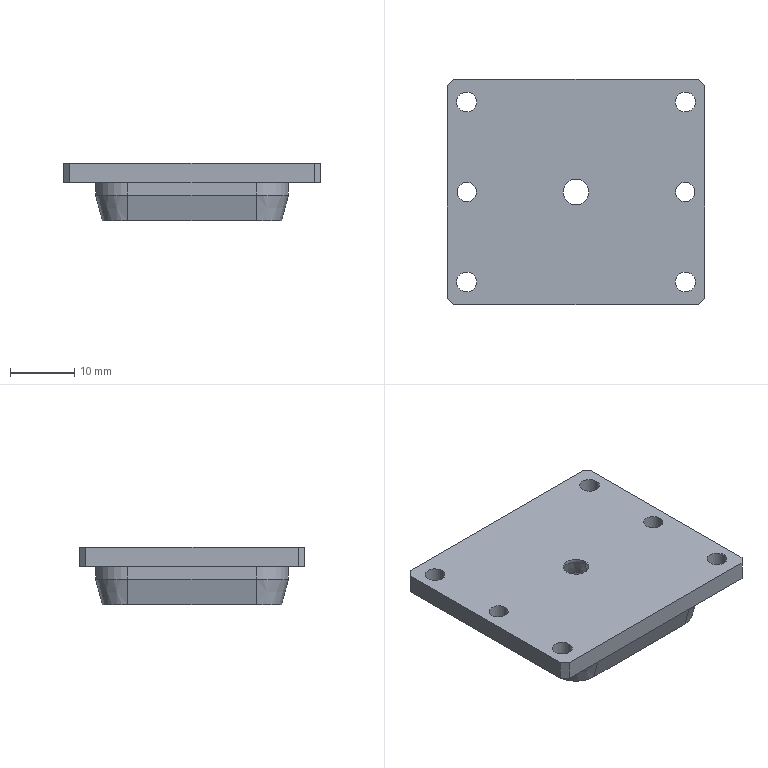Part | NX | features BREP 1 | 1 solid | 46 faces | box 40 x 35 x 9 mm | volume 6971 mm3 | cylinder 20 | plane 20 | cone 6 | commonest cylinder face diameters 3.1 x8 3 x4 10 x4 4 x2 21 x2
STEP:
#1=CARTESIAN_POINT('',(2.,0.,1.));
#2=VERTEX_POINT('',#1);
#3=CARTESIAN_POINT('',(-2.,0.,1.));
#4=VERTEX_POINT('',#3);
#5=CARTESIAN_POINT('',(0.,0.,1.));
#6=DIRECTION('',(0.,0.,-1.));
#7=DIRECTION('',(-1.,0.,0.));
#8=AXIS2_PLACEMENT_3D('',#5,#6,#7);
#9=CIRCLE('',#8,2.);
#10=EDGE_CURVE('',#2,#4,#9,.T.);
#11=ORIENTED_EDGE('',*,*,#10,.F.);
#12=CARTESIAN_POINT('',(2.67,0.,-1.5));
#13=VERTEX_POINT('',#12);
#14=CARTESIAN_POINT('',(2.67,0.,-1.5));
#15=DIRECTION('',(0.2588,0.,-0.9659));
#16=VECTOR('',#15,1000.);
#17=LINE('',#14,#16);
#18=EDGE_CURVE('',#2,#13,#17,.T.);
#19=ORIENTED_EDGE('',*,*,#18,.T.);
#20=CARTESIAN_POINT('',(-2.67,0.,-1.5));
#21=VERTEX_POINT('',#20);
#22=CARTESIAN_POINT('',(0.,0.,-1.5));
#23=DIRECTION('',(0.,0.,1.));
#24=DIRECTION('',(-1.,0.,0.));
#25=AXIS2_PLACEMENT_3D('',#22,#23,#24);
#26=CIRCLE('',#25,2.67);
#27=EDGE_CURVE('',#21,#13,#26,.T.);
#28=ORIENTED_EDGE('',*,*,#27,.F.);
#29=CARTESIAN_POINT('',(-2.67,0.,-1.5));
#30=DIRECTION('',(-0.2588,0.,-0.9659));
#31=VECTOR('',#30,1000.);
#32=LINE('',#29,#31);
#33=EDGE_CURVE('',#4,#21,#32,.T.);
#34=ORIENTED_EDGE('',*,*,#33,.F.);
#35=EDGE_LOOP('',(#11,#19,#28,#34));
#36=FACE_BOUND('',#35,.T.);
#37=CARTESIAN_POINT('',(0.,0.,-1.5));
#38=DIRECTION('',(0.,0.,-1.));
#39=DIRECTION('',(-1.,0.,0.));
#40=AXIS2_PLACEMENT_3D('',#37,#38,#39);
#41=CONICAL_SURFACE('',#40,2.67,0.2618);
#42=ADVANCED_FACE('',(#36),#41,.F.);
#43=CARTESIAN_POINT('',(10.5,0.,-1.5));
#44=VERTEX_POINT('',#43);
#45=CARTESIAN_POINT('',(-10.5,0.,-1.5));
#46=VERTEX_POINT('',#45);
#47=CARTESIAN_POINT('',(0.,0.,-1.5));
#48=DIRECTION('',(0.,0.,-1.));
#49=DIRECTION('',(-1.,0.,0.));
#50=AXIS2_PLACEMENT_3D('',#47,#48,#49);
#51=CIRCLE('',#50,10.5);
#52=EDGE_CURVE('',#44,#46,#51,.T.);
#53=ORIENTED_EDGE('',*,*,#52,.F.);
#54=CARTESIAN_POINT('',(10.5,0.,-7.5));
#55=VERTEX_POINT('',#54);
#56=CARTESIAN_POINT('',(10.5,0.,-1.5));
#57=DIRECTION('',(0.,0.,-1.));
#58=VECTOR('',#57,1000.);
#59=LINE('',#56,#58);
#60=EDGE_CURVE('',#44,#55,#59,.T.);
#61=ORIENTED_EDGE('',*,*,#60,.T.);
#62=CARTESIAN_POINT('',(-10.5,0.,-7.5));
#63=VERTEX_POINT('',#62);
#64=CARTESIAN_POINT('',(0.,0.,-7.5));
#65=DIRECTION('',(0.,0.,-1.));
#66=DIRECTION('',(-1.,0.,0.));
#67=AXIS2_PLACEMENT_3D('',#64,#65,#66);
#68=CIRCLE('',#67,10.5);
#69=EDGE_CURVE('',#55,#63,#68,.T.);
#70=ORIENTED_EDGE('',*,*,#69,.T.);
#71=CARTESIAN_POINT('',(-10.5,0.,-1.5));
#72=DIRECTION('',(0.,0.,-1.));
#73=VECTOR('',#72,1000.);
#74=LINE('',#71,#73);
#75=EDGE_CURVE('',#46,#63,#74,.T.);
#76=ORIENTED_EDGE('',*,*,#75,.F.);
#77=EDGE_LOOP('',(#53,#61,#70,#76));
#78=FACE_BOUND('',#77,.T.);
#79=CARTESIAN_POINT('',(0.,0.,-1.5));
#80=DIRECTION('',(0.,0.,-1.));
#81=DIRECTION('',(-1.,0.,0.));
#82=AXIS2_PLACEMENT_3D('',#79,#80,#81);
#83=CYLINDRICAL_SURFACE('',#82,10.5);
#84=ADVANCED_FACE('',(#78),#83,.F.);
#85=CARTESIAN_POINT('',(-18.55,14.,-1.5));
#86=VERTEX_POINT('',#85);
#87=CARTESIAN_POINT('',(-15.45,14.,-1.5));
#88=VERTEX_POINT('',#87);
#89=CARTESIAN_POINT('',(-17.,14.,-1.5));
#90=DIRECTION('',(0.,0.,1.));
#91=DIRECTION('',(1.,0.,0.));
#92=AXIS2_PLACEMENT_3D('',#89,#90,#91);
#93=CIRCLE('',#92,1.55);
#94=EDGE_CURVE('',#86,#88,#93,.T.);
#95=ORIENTED_EDGE('',*,*,#94,.F.);
#96=CARTESIAN_POINT('',(-18.55,14.,1.5));
#97=VERTEX_POINT('',#96);
#98=CARTESIAN_POINT('',(-18.55,14.,1.5));
#99=DIRECTION('',(0.,0.,1.));
#100=VECTOR('',#99,1000.);
#101=LINE('',#98,#100);
#102=EDGE_CURVE('',#97,#86,#101,.F.);
#103=ORIENTED_EDGE('',*,*,#102,.F.);
#104=CARTESIAN_POINT('',(-15.45,14.,1.5));
#105=VERTEX_POINT('',#104);
#106=CARTESIAN_POINT('',(-17.,14.,1.5));
#107=DIRECTION('',(0.,0.,1.));
#108=DIRECTION('',(1.,0.,0.));
#109=AXIS2_PLACEMENT_3D('',#106,#107,#108);
#110=CIRCLE('',#109,1.55);
#111=EDGE_CURVE('',#97,#105,#110,.T.);
#112=ORIENTED_EDGE('',*,*,#111,.T.);
#113=CARTESIAN_POINT('',(-15.45,14.,1.5));
#114=DIRECTION('',(0.,0.,1.));
#115=VECTOR('',#114,1000.);
#116=LINE('',#113,#115);
#117=EDGE_CURVE('',#105,#88,#116,.F.);
#118=ORIENTED_EDGE('',*,*,#117,.T.);
#119=EDGE_LOOP('',(#95,#103,#112,#118));
#120=FACE_BOUND('',#119,.T.);
#121=CARTESIAN_POINT('',(-17.,14.,1.5));
#122=DIRECTION('',(0.,0.,1.));
#123=DIRECTION('',(1.,0.,0.));
#124=AXIS2_PLACEMENT_3D('',#121,#122,#123);
#125=CYLINDRICAL_SURFACE('',#124,1.55);
#126=ADVANCED_FACE('',(#120),#125,.F.);
#127=CARTESIAN_POINT('',(-18.55,-14.,-1.5));
#128=VERTEX_POINT('',#127);
#129=CARTESIAN_POINT('',(-15.45,-14.,-1.5));
#130=VERTEX_POINT('',#129);
#131=CARTESIAN_POINT('',(-17.,-14.,-1.5));
#132=DIRECTION('',(0.,0.,1.));
#133=DIRECTION('',(1.,0.,0.));
#134=AXIS2_PLACEMENT_3D('',#131,#132,#133);
#135=CIRCLE('',#134,1.55);
#136=EDGE_CURVE('',#128,#130,#135,.T.);
#137=ORIENTED_EDGE('',*,*,#136,.F.);
#138=CARTESIAN_POINT('',(-18.55,-14.,1.5));
#139=VERTEX_POINT('',#138);
#140=CARTESIAN_POINT('',(-18.55,-14.,1.5));
#141=DIRECTION('',(0.,0.,1.));
#142=VECTOR('',#141,1000.);
#143=LINE('',#140,#142);
#144=EDGE_CURVE('',#139,#128,#143,.F.);
#145=ORIENTED_EDGE('',*,*,#144,.F.);
#146=CARTESIAN_POINT('',(-15.45,-14.,1.5));
#147=VERTEX_POINT('',#146);
#148=CARTESIAN_POINT('',(-17.,-14.,1.5));
#149=DIRECTION('',(0.,0.,1.));
#150=DIRECTION('',(1.,0.,0.));
#151=AXIS2_PLACEMENT_3D('',#148,#149,#150);
#152=CIRCLE('',#151,1.55);
#153=EDGE_CURVE('',#139,#147,#152,.T.);
#154=ORIENTED_EDGE('',*,*,#153,.T.);
#155=CARTESIAN_POINT('',(-15.45,-14.,1.5));
#156=DIRECTION('',(0.,0.,1.));
#157=VECTOR('',#156,1000.);
#158=LINE('',#155,#157);
#159=EDGE_CURVE('',#147,#130,#158,.F.);
#160=ORIENTED_EDGE('',*,*,#159,.T.);
#161=EDGE_LOOP('',(#137,#145,#154,#160));
#162=FACE_BOUND('',#161,.T.);
#163=CARTESIAN_POINT('',(-17.,-14.,1.5));
#164=DIRECTION('',(0.,0.,1.));
#165=DIRECTION('',(1.,0.,0.));
#166=AXIS2_PLACEMENT_3D('',#163,#164,#165);
#167=CYLINDRICAL_SURFACE('',#166,1.55);
#168=ADVANCED_FACE('',(#162),#167,.F.);
#169=CARTESIAN_POINT('',(15.45,-14.,-1.5));
#170=VERTEX_POINT('',#169);
#171=CARTESIAN_POINT('',(18.55,-14.,-1.5));
#172=VERTEX_POINT('',#171);
#173=CARTESIAN_POINT('',(17.,-14.,-1.5));
#174=DIRECTION('',(0.,0.,1.));
#175=DIRECTION('',(1.,0.,0.));
#176=AXIS2_PLACEMENT_3D('',#173,#174,#175);
#177=CIRCLE('',#176,1.55);
#178=EDGE_CURVE('',#170,#172,#177,.T.);
#179=ORIENTED_EDGE('',*,*,#178,.F.);
#180=CARTESIAN_POINT('',(15.45,-14.,1.5));
#181=VERTEX_POINT('',#180);
#182=CARTESIAN_POINT('',(15.45,-14.,1.5));
#183=DIRECTION('',(0.,0.,1.));
#184=VECTOR('',#183,1000.);
#185=LINE('',#182,#184);
#186=EDGE_CURVE('',#181,#170,#185,.F.);
#187=ORIENTED_EDGE('',*,*,#186,.F.);
#188=CARTESIAN_POINT('',(18.55,-14.,1.5));
#189=VERTEX_POINT('',#188);
#190=CARTESIAN_POINT('',(17.,-14.,1.5));
#191=DIRECTION('',(0.,0.,1.));
#192=DIRECTION('',(1.,0.,0.));
#193=AXIS2_PLACEMENT_3D('',#190,#191,#192);
#194=CIRCLE('',#193,1.55);
#195=EDGE_CURVE('',#181,#189,#194,.T.);
#196=ORIENTED_EDGE('',*,*,#195,.T.);
#197=CARTESIAN_POINT('',(18.55,-14.,1.5));
#198=DIRECTION('',(0.,0.,1.));
#199=VECTOR('',#198,1000.);
#200=LINE('',#197,#199);
#201=EDGE_CURVE('',#189,#172,#200,.F.);
#202=ORIENTED_EDGE('',*,*,#201,.T.);
#203=EDGE_LOOP('',(#179,#187,#196,#202));
#204=FACE_BOUND('',#203,.T.);
#205=CARTESIAN_POINT('',(17.,-14.,1.5));
#206=DIRECTION('',(0.,0.,1.));
#207=DIRECTION('',(1.,0.,0.));
#208=AXIS2_PLACEMENT_3D('',#205,#206,#207);
#209=CYLINDRICAL_SURFACE('',#208,1.55);
#210=ADVANCED_FACE('',(#204),#209,.F.);
#211=CARTESIAN_POINT('',(15.45,14.,-1.5));
#212=VERTEX_POINT('',#211);
#213=CARTESIAN_POINT('',(18.55,14.,-1.5));
#214=VERTEX_POINT('',#213);
#215=CARTESIAN_POINT('',(17.,14.,-1.5));
#216=DIRECTION('',(0.,0.,1.));
#217=DIRECTION('',(1.,0.,0.));
#218=AXIS2_PLACEMENT_3D('',#215,#216,#217);
#219=CIRCLE('',#218,1.55);
#220=EDGE_CURVE('',#212,#214,#219,.T.);
#221=ORIENTED_EDGE('',*,*,#220,.F.);
#222=CARTESIAN_POINT('',(15.45,14.,1.5));
#223=VERTEX_POINT('',#222);
#224=CARTESIAN_POINT('',(15.45,14.,1.5));
#225=DIRECTION('',(0.,0.,1.));
#226=VECTOR('',#225,1000.);
#227=LINE('',#224,#226);
#228=EDGE_CURVE('',#223,#212,#227,.F.);
#229=ORIENTED_EDGE('',*,*,#228,.F.);
#230=CARTESIAN_POINT('',(18.55,14.,1.5));
#231=VERTEX_POINT('',#230);
#232=CARTESIAN_POINT('',(17.,14.,1.5));
#233=DIRECTION('',(0.,0.,1.));
#234=DIRECTION('',(1.,0.,0.));
#235=AXIS2_PLACEMENT_3D('',#232,#233,#234);
#236=CIRCLE('',#235,1.55);
#237=EDGE_CURVE('',#223,#231,#236,.T.);
#238=ORIENTED_EDGE('',*,*,#237,.T.);
#239=CARTESIAN_POINT('',(18.55,14.,1.5));
#240=DIRECTION('',(0.,0.,1.));
#241=VECTOR('',#240,1000.);
#242=LINE('',#239,#241);
#243=EDGE_CURVE('',#231,#214,#242,.F.);
#244=ORIENTED_EDGE('',*,*,#243,.T.);
#245=EDGE_LOOP('',(#221,#229,#238,#244));
#246=FACE_BOUND('',#245,.T.);
#247=CARTESIAN_POINT('',(17.,14.,1.5));
#248=DIRECTION('',(0.,0.,1.));
#249=DIRECTION('',(1.,0.,0.));
#250=AXIS2_PLACEMENT_3D('',#247,#248,#249);
#251=CYLINDRICAL_SURFACE('',#250,1.55);
#252=ADVANCED_FACE('',(#246),#251,.F.);
#253=CARTESIAN_POINT('',(-18.5,0.,-1.5));
#254=VERTEX_POINT('',#253);
#255=CARTESIAN_POINT('',(-15.5,0.,-1.5));
#256=VERTEX_POINT('',#255);
#257=CARTESIAN_POINT('',(-17.,0.,-1.5));
#258=DIRECTION('',(0.,0.,1.));
#259=DIRECTION('',(1.,0.,0.));
#260=AXIS2_PLACEMENT_3D('',#257,#258,#259);
#261=CIRCLE('',#260,1.5);
#262=EDGE_CURVE('',#254,#256,#261,.T.);
#263=ORIENTED_EDGE('',*,*,#262,.F.);
#264=CARTESIAN_POINT('',(-18.5,0.,1.5));
#265=VERTEX_POINT('',#264);
#266=CARTESIAN_POINT('',(-18.5,0.,-7.5));
#267=DIRECTION('',(0.,0.,1.));
#268=VECTOR('',#267,1000.);
#269=LINE('',#266,#268);
#270=EDGE_CURVE('',#265,#254,#269,.F.);
#271=ORIENTED_EDGE('',*,*,#270,.F.);
#272=CARTESIAN_POINT('',(-15.5,0.,1.5));
#273=VERTEX_POINT('',#272);
#274=CARTESIAN_POINT('',(-17.,0.,1.5));
#275=DIRECTION('',(0.,0.,1.));
#276=DIRECTION('',(1.,0.,0.));
#277=AXIS2_PLACEMENT_3D('',#274,#275,#276);
#278=CIRCLE('',#277,1.5);
#279=EDGE_CURVE('',#265,#273,#278,.T.);
#280=ORIENTED_EDGE('',*,*,#279,.T.);
#281=CARTESIAN_POINT('',(-15.5,0.,-7.5));
#282=DIRECTION('',(0.,0.,1.));
#283=VECTOR('',#282,1000.);
#284=LINE('',#281,#283);
#285=EDGE_CURVE('',#273,#256,#284,.F.);
#286=ORIENTED_EDGE('',*,*,#285,.T.);
#287=EDGE_LOOP('',(#263,#271,#280,#286));
#288=FACE_BOUND('',#287,.T.);
#289=CARTESIAN_POINT('',(-17.,0.,-7.5));
#290=DIRECTION('',(0.,0.,1.));
#291=DIRECTION('',(1.,0.,0.));
#292=AXIS2_PLACEMENT_3D('',#289,#290,#291);
#293=CYLINDRICAL_SURFACE('',#292,1.5);
#294=ADVANCED_FACE('',(#288),#293,.F.);
#295=CARTESIAN_POINT('',(15.5,0.,-1.5));
#296=VERTEX_POINT('',#295);
#297=CARTESIAN_POINT('',(18.5,0.,-1.5));
#298=VERTEX_POINT('',#297);
#299=CARTESIAN_POINT('',(17.,0.,-1.5));
#300=DIRECTION('',(0.,0.,1.));
#301=DIRECTION('',(1.,0.,0.));
#302=AXIS2_PLACEMENT_3D('',#299,#300,#301);
#303=CIRCLE('',#302,1.5);
#304=EDGE_CURVE('',#296,#298,#303,.T.);
#305=ORIENTED_EDGE('',*,*,#304,.F.);
#306=CARTESIAN_POINT('',(15.5,0.,1.5));
#307=VERTEX_POINT('',#306);
#308=CARTESIAN_POINT('',(15.5,0.,-7.5));
#309=DIRECTION('',(0.,0.,1.));
#310=VECTOR('',#309,1000.);
#311=LINE('',#308,#310);
#312=EDGE_CURVE('',#307,#296,#311,.F.);
#313=ORIENTED_EDGE('',*,*,#312,.F.);
#314=CARTESIAN_POINT('',(18.5,0.,1.5));
#315=VERTEX_POINT('',#314);
#316=CARTESIAN_POINT('',(17.,0.,1.5));
#317=DIRECTION('',(0.,0.,1.));
#318=DIRECTION('',(1.,0.,0.));
#319=AXIS2_PLACEMENT_3D('',#316,#317,#318);
#320=CIRCLE('',#319,1.5);
#321=EDGE_CURVE('',#307,#315,#320,.T.);
#322=ORIENTED_EDGE('',*,*,#321,.T.);
#323=CARTESIAN_POINT('',(18.5,0.,-7.5));
#324=DIRECTION('',(0.,0.,1.));
#325=VECTOR('',#324,1000.);
#326=LINE('',#323,#325);
#327=EDGE_CURVE('',#315,#298,#326,.F.);
#328=ORIENTED_EDGE('',*,*,#327,.T.);
#329=EDGE_LOOP('',(#305,#313,#322,#328));
#330=FACE_BOUND('',#329,.T.);
#331=CARTESIAN_POINT('',(17.,0.,-7.5));
#332=DIRECTION('',(0.,0.,1.));
#333=DIRECTION('',(1.,0.,0.));
#334=AXIS2_PLACEMENT_3D('',#331,#332,#333);
#335=CYLINDRICAL_SURFACE('',#334,1.5);
#336=ADVANCED_FACE('',(#330),#335,.F.);
#337=ORIENTED_EDGE('',*,*,#10,.T.);
#338=CARTESIAN_POINT('',(-2.,0.,1.5));
#339=VERTEX_POINT('',#338);
#340=CARTESIAN_POINT('',(-2.,0.,-7.5));
#341=DIRECTION('',(0.,0.,1.));
#342=VECTOR('',#341,1000.);
#343=LINE('',#340,#342);
#344=EDGE_CURVE('',#339,#4,#343,.F.);
#345=ORIENTED_EDGE('',*,*,#344,.F.);
#346=CARTESIAN_POINT('',(2.,0.,1.5));
#347=VERTEX_POINT('',#346);
#348=CARTESIAN_POINT('',(0.,0.,1.5));
#349=DIRECTION('',(0.,0.,1.));
#350=DIRECTION('',(1.,0.,0.));
#351=AXIS2_PLACEMENT_3D('',#348,#349,#350);
#352=CIRCLE('',#351,2.);
#353=EDGE_CURVE('',#339,#347,#352,.T.);
#354=ORIENTED_EDGE('',*,*,#353,.T.);
#355=CARTESIAN_POINT('',(2.,0.,-7.5));
#356=DIRECTION('',(0.,0.,1.));
#357=VECTOR('',#356,1000.);
#358=LINE('',#355,#357);
#359=EDGE_CURVE('',#347,#2,#358,.F.);
#360=ORIENTED_EDGE('',*,*,#359,.T.);
#361=EDGE_LOOP('',(#337,#345,#354,#360));
#362=FACE_BOUND('',#361,.T.);
#363=CARTESIAN_POINT('',(0.,0.,-7.5));
#364=DIRECTION('',(0.,0.,1.));
#365=DIRECTION('',(1.,0.,0.));
#366=AXIS2_PLACEMENT_3D('',#363,#364,#365);
#367=CYLINDRICAL_SURFACE('',#366,2.);
#368=ADVANCED_FACE('',(#362),#367,.F.);
#369=ORIENTED_EDGE('',*,*,#344,.T.);
#370=CARTESIAN_POINT('',(0.,0.,1.));
#371=DIRECTION('',(0.,0.,-1.));
#372=DIRECTION('',(-1.,0.,0.));
#373=AXIS2_PLACEMENT_3D('',#370,#371,#372);
#374=CIRCLE('',#373,2.);
#375=EDGE_CURVE('',#4,#2,#374,.T.);
#376=ORIENTED_EDGE('',*,*,#375,.T.);
#377=ORIENTED_EDGE('',*,*,#359,.F.);
#378=CARTESIAN_POINT('',(0.,0.,1.5));
#379=DIRECTION('',(0.,0.,1.));
#380=DIRECTION('',(1.,0.,0.));
#381=AXIS2_PLACEMENT_3D('',#378,#379,#380);
#382=CIRCLE('',#381,2.);
#383=EDGE_CURVE('',#347,#339,#382,.T.);
#384=ORIENTED_EDGE('',*,*,#383,.T.);
#385=EDGE_LOOP('',(#369,#376,#377,#384));
#386=FACE_BOUND('',#385,.T.);
#387=CARTESIAN_POINT('',(0.,0.,-7.5));
#388=DIRECTION('',(0.,0.,1.));
#389=DIRECTION('',(1.,0.,0.));
#390=AXIS2_PLACEMENT_3D('',#387,#388,#389);
#391=CYLINDRICAL_SURFACE('',#390,2.);
#392=ADVANCED_FACE('',(#386),#391,.F.);
#393=CARTESIAN_POINT('',(-20.,16.5,-1.5));
#394=VERTEX_POINT('',#393);
#395=CARTESIAN_POINT('',(-20.,-16.5,-1.5));
#396=VERTEX_POINT('',#395);
#397=CARTESIAN_POINT('',(-20.,-17.5,-1.5));
#398=DIRECTION('',(0.,-1.,0.));
#399=VECTOR('',#398,1000.);
#400=LINE('',#397,#399);
#401=EDGE_CURVE('',#394,#396,#400,.T.);
#402=ORIENTED_EDGE('',*,*,#401,.T.);
#403=CARTESIAN_POINT('',(-20.,-16.5,1.5));
#404=VERTEX_POINT('',#403);
#405=CARTESIAN_POINT('',(-20.,-16.5,1.5));
#406=DIRECTION('',(0.,0.,1.));
#407=VECTOR('',#406,1000.);
#408=LINE('',#405,#407);
#409=EDGE_CURVE('',#396,#404,#408,.T.);
#410=ORIENTED_EDGE('',*,*,#409,.T.);
#411=CARTESIAN_POINT('',(-20.,16.5,1.5));
#412=VERTEX_POINT('',#411);
#413=CARTESIAN_POINT('',(-20.,-17.5,1.5));
#414=DIRECTION('',(0.,-1.,0.));
#415=VECTOR('',#414,1000.);
#416=LINE('',#413,#415);
#417=EDGE_CURVE('',#412,#404,#416,.T.);
#418=ORIENTED_EDGE('',*,*,#417,.F.);
#419=CARTESIAN_POINT('',(-20.,16.5,1.5));
#420=DIRECTION('',(0.,0.,-1.));
#421=VECTOR('',#420,1000.);
#422=LINE('',#419,#421);
#423=EDGE_CURVE('',#412,#394,#422,.T.);
#424=ORIENTED_EDGE('',*,*,#423,.T.);
#425=EDGE_LOOP('',(#402,#410,#418,#424));
#426=FACE_BOUND('',#425,.T.);
#427=CARTESIAN_POINT('',(-20.,-17.5,1.5));
#428=DIRECTION('',(1.,0.,0.));
#429=DIRECTION('',(0.,1.,0.));
#430=AXIS2_PLACEMENT_3D('',#427,#428,#429);
#431=PLANE('',#430);
#432=ADVANCED_FACE('',(#426),#431,.F.);
#433=CARTESIAN_POINT('',(-19.,-17.5,-1.5));
#434=VERTEX_POINT('',#433);
#435=CARTESIAN_POINT('',(19.,-17.5,-1.5));
#436=VERTEX_POINT('',#435);
#437=CARTESIAN_POINT('',(20.,-17.5,-1.5));
#438=DIRECTION('',(1.,0.,0.));
#439=VECTOR('',#438,1000.);
#440=LINE('',#437,#439);
#441=EDGE_CURVE('',#434,#436,#440,.T.);
#442=ORIENTED_EDGE('',*,*,#441,.T.);
#443=CARTESIAN_POINT('',(19.,-17.5,1.5));
#444=VERTEX_POINT('',#443);
#445=CARTESIAN_POINT('',(19.,-17.5,1.5));
#446=DIRECTION('',(0.,0.,1.));
#447=VECTOR('',#446,1000.);
#448=LINE('',#445,#447);
#449=EDGE_CURVE('',#436,#444,#448,.T.);
#450=ORIENTED_EDGE('',*,*,#449,.T.);
#451=CARTESIAN_POINT('',(-19.,-17.5,1.5));
#452=VERTEX_POINT('',#451);
#453=CARTESIAN_POINT('',(20.,-17.5,1.5));
#454=DIRECTION('',(1.,0.,0.));
#455=VECTOR('',#454,1000.);
#456=LINE('',#453,#455);
#457=EDGE_CURVE('',#452,#444,#456,.T.);
#458=ORIENTED_EDGE('',*,*,#457,.F.);
#459=CARTESIAN_POINT('',(-19.,-17.5,1.5));
#460=DIRECTION('',(0.,0.,-1.));
#461=VECTOR('',#460,1000.);
#462=LINE('',#459,#461);
#463=EDGE_CURVE('',#452,#434,#462,.T.);
#464=ORIENTED_EDGE('',*,*,#463,.T.);
#465=EDGE_LOOP('',(#442,#450,#458,#464));
#466=FACE_BOUND('',#465,.T.);
#467=CARTESIAN_POINT('',(20.,-17.5,1.5));
#468=DIRECTION('',(0.,1.,0.));
#469=DIRECTION('',(1.,0.,0.));
#470=AXIS2_PLACEMENT_3D('',#467,#468,#469);
#471=PLANE('',#470);
#472=ADVANCED_FACE('',(#466),#471,.F.);
#473=CARTESIAN_POINT('',(20.,-16.5,1.5));
#474=VERTEX_POINT('',#473);
#475=CARTESIAN_POINT('',(20.,16.5,1.5));
#476=VERTEX_POINT('',#475);
#477=CARTESIAN_POINT('',(20.,-17.5,1.5));
#478=DIRECTION('',(0.,1.,0.));
#479=VECTOR('',#478,1000.);
#480=LINE('',#477,#479);
#481=EDGE_CURVE('',#474,#476,#480,.T.);
#482=ORIENTED_EDGE('',*,*,#481,.F.);
#483=CARTESIAN_POINT('',(20.,-16.5,-1.5));
#484=VERTEX_POINT('',#483);
#485=CARTESIAN_POINT('',(20.,-16.5,1.5));
#486=DIRECTION('',(0.,0.,-1.));
#487=VECTOR('',#486,1000.);
#488=LINE('',#485,#487);
#489=EDGE_CURVE('',#474,#484,#488,.T.);
#490=ORIENTED_EDGE('',*,*,#489,.T.);
#491=CARTESIAN_POINT('',(20.,16.5,-1.5));
#492=VERTEX_POINT('',#491);
#493=CARTESIAN_POINT('',(20.,-17.5,-1.5));
#494=DIRECTION('',(0.,1.,0.));
#495=VECTOR('',#494,1000.);
#496=LINE('',#493,#495);
#497=EDGE_CURVE('',#484,#492,#496,.T.);
#498=ORIENTED_EDGE('',*,*,#497,.T.);
#499=CARTESIAN_POINT('',(20.,16.5,1.5));
#500=DIRECTION('',(0.,0.,1.));
#501=VECTOR('',#500,1000.);
#502=LINE('',#499,#501);
#503=EDGE_CURVE('',#492,#476,#502,.T.);
#504=ORIENTED_EDGE('',*,*,#503,.T.);
#505=EDGE_LOOP('',(#482,#490,#498,#504));
#506=FACE_BOUND('',#505,.T.);
#507=CARTESIAN_POINT('',(20.,-17.5,1.5));
#508=DIRECTION('',(-1.,0.,0.));
#509=DIRECTION('',(0.,0.,1.));
#510=AXIS2_PLACEMENT_3D('',#507,#508,#509);
#511=PLANE('',#510);
#512=ADVANCED_FACE('',(#506),#511,.F.);
#513=CARTESIAN_POINT('',(19.,17.5,1.5));
#514=VERTEX_POINT('',#513);
#515=CARTESIAN_POINT('',(-19.,17.5,1.5));
#516=VERTEX_POINT('',#515);
#517=CARTESIAN_POINT('',(20.,17.5,1.5));
#518=DIRECTION('',(-1.,0.,0.));
#519=VECTOR('',#518,1000.);
#520=LINE('',#517,#519);
#521=EDGE_CURVE('',#514,#516,#520,.T.);
#522=ORIENTED_EDGE('',*,*,#521,.F.);
#523=CARTESIAN_POINT('',(19.,17.5,-1.5));
#524=VERTEX_POINT('',#523);
#525=CARTESIAN_POINT('',(19.,17.5,1.5));
#526=DIRECTION('',(0.,0.,-1.));
#527=VECTOR('',#526,1000.);
#528=LINE('',#525,#527);
#529=EDGE_CURVE('',#514,#524,#528,.T.);
#530=ORIENTED_EDGE('',*,*,#529,.T.);
#531=CARTESIAN_POINT('',(-19.,17.5,-1.5));
#532=VERTEX_POINT('',#531);
#533=CARTESIAN_POINT('',(20.,17.5,-1.5));
#534=DIRECTION('',(-1.,0.,0.));
#535=VECTOR('',#534,1000.);
#536=LINE('',#533,#535);
#537=EDGE_CURVE('',#524,#532,#536,.T.);
#538=ORIENTED_EDGE('',*,*,#537,.T.);
#539=CARTESIAN_POINT('',(-19.,17.5,1.5));
#540=DIRECTION('',(0.,0.,1.));
#541=VECTOR('',#540,1000.);
#542=LINE('',#539,#541);
#543=EDGE_CURVE('',#532,#516,#542,.T.);
#544=ORIENTED_EDGE('',*,*,#543,.T.);
#545=EDGE_LOOP('',(#522,#530,#538,#544));
#546=FACE_BOUND('',#545,.T.);
#547=CARTESIAN_POINT('',(20.,17.5,1.5));
#548=DIRECTION('',(0.,-1.,0.));
#549=DIRECTION('',(0.,0.,-1.));
#550=AXIS2_PLACEMENT_3D('',#547,#548,#549);
#551=PLANE('',#550);
#552=ADVANCED_FACE('',(#546),#551,.F.);
#553=ORIENTED_EDGE('',*,*,#457,.T.);
#554=CARTESIAN_POINT('',(18.25,-18.25,1.5));
#555=DIRECTION('',(0.7071,0.7071,0.));
#556=VECTOR('',#555,1000.);
#557=LINE('',#554,#556);
#558=EDGE_CURVE('',#444,#474,#557,.T.);
#559=ORIENTED_EDGE('',*,*,#558,.T.);
#560=ORIENTED_EDGE('',*,*,#481,.T.);
#561=CARTESIAN_POINT('',(18.25,18.25,1.5));
#562=DIRECTION('',(-0.7071,0.7071,0.));
#563=VECTOR('',#562,1000.);
#564=LINE('',#561,#563);
#565=EDGE_CURVE('',#476,#514,#564,.T.);
#566=ORIENTED_EDGE('',*,*,#565,.T.);
#567=ORIENTED_EDGE('',*,*,#521,.T.);
#568=CARTESIAN_POINT('',(-18.25,18.25,1.5));
#569=DIRECTION('',(-0.7071,-0.7071,0.));
#570=VECTOR('',#569,1000.);
#571=LINE('',#568,#570);
#572=EDGE_CURVE('',#516,#412,#571,.T.);
#573=ORIENTED_EDGE('',*,*,#572,.T.);
#574=ORIENTED_EDGE('',*,*,#417,.T.);
#575=CARTESIAN_POINT('',(-18.25,-18.25,1.5));
#576=DIRECTION('',(0.7071,-0.7071,0.));
#577=VECTOR('',#576,1000.);
#578=LINE('',#575,#577);
#579=EDGE_CURVE('',#404,#452,#578,.T.);
#580=ORIENTED_EDGE('',*,*,#579,.T.);
#581=EDGE_LOOP('',(#553,#559,#560,#566,#567,#573,#574,#580));
#582=FACE_BOUND('',#581,.T.);
#583=ORIENTED_EDGE('',*,*,#383,.F.);
#584=ORIENTED_EDGE('',*,*,#353,.F.);
#585=EDGE_LOOP('',(#583,#584));
#586=FACE_BOUND('',#585,.T.);
#587=CARTESIAN_POINT('',(-17.,14.,1.5));
#588=DIRECTION('',(0.,0.,1.));
#589=DIRECTION('',(1.,0.,0.));
#590=AXIS2_PLACEMENT_3D('',#587,#588,#589);
#591=CIRCLE('',#590,1.55);
#592=EDGE_CURVE('',#105,#97,#591,.T.);
#593=ORIENTED_EDGE('',*,*,#592,.F.);
#594=ORIENTED_EDGE('',*,*,#111,.F.);
#595=EDGE_LOOP('',(#593,#594));
#596=FACE_BOUND('',#595,.T.);
#597=CARTESIAN_POINT('',(-17.,-14.,1.5));
#598=DIRECTION('',(0.,0.,1.));
#599=DIRECTION('',(1.,0.,0.));
#600=AXIS2_PLACEMENT_3D('',#597,#598,#599);
#601=CIRCLE('',#600,1.55);
#602=EDGE_CURVE('',#147,#139,#601,.T.);
#603=ORIENTED_EDGE('',*,*,#602,.F.);
#604=ORIENTED_EDGE('',*,*,#153,.F.);
#605=EDGE_LOOP('',(#603,#604));
#606=FACE_BOUND('',#605,.T.);
#607=CARTESIAN_POINT('',(17.,-14.,1.5));
#608=DIRECTION('',(0.,0.,1.));
#609=DIRECTION('',(1.,0.,0.));
#610=AXIS2_PLACEMENT_3D('',#607,#608,#609);
#611=CIRCLE('',#610,1.55);
#612=EDGE_CURVE('',#189,#181,#611,.T.);
#613=ORIENTED_EDGE('',*,*,#612,.F.);
#614=ORIENTED_EDGE('',*,*,#195,.F.);
#615=EDGE_LOOP('',(#613,#614));
#616=FACE_BOUND('',#615,.T.);
#617=CARTESIAN_POINT('',(17.,14.,1.5));
#618=DIRECTION('',(0.,0.,1.));
#619=DIRECTION('',(1.,0.,0.));
#620=AXIS2_PLACEMENT_3D('',#617,#618,#619);
#621=CIRCLE('',#620,1.55);
#622=EDGE_CURVE('',#231,#223,#621,.T.);
#623=ORIENTED_EDGE('',*,*,#622,.F.);
#624=ORIENTED_EDGE('',*,*,#237,.F.);
#625=EDGE_LOOP('',(#623,#624));
#626=FACE_BOUND('',#625,.T.);
#627=CARTESIAN_POINT('',(-17.,0.,1.5));
#628=DIRECTION('',(0.,0.,1.));
#629=DIRECTION('',(1.,0.,0.));
#630=AXIS2_PLACEMENT_3D('',#627,#628,#629);
#631=CIRCLE('',#630,1.5);
#632=EDGE_CURVE('',#273,#265,#631,.T.);
#633=ORIENTED_EDGE('',*,*,#632,.F.);
#634=ORIENTED_EDGE('',*,*,#279,.F.);
#635=EDGE_LOOP('',(#633,#634));
#636=FACE_BOUND('',#635,.T.);
#637=CARTESIAN_POINT('',(17.,0.,1.5));
#638=DIRECTION('',(0.,0.,1.));
#639=DIRECTION('',(1.,0.,0.));
#640=AXIS2_PLACEMENT_3D('',#637,#638,#639);
#641=CIRCLE('',#640,1.5);
#642=EDGE_CURVE('',#315,#307,#641,.T.);
#643=ORIENTED_EDGE('',*,*,#642,.F.);
#644=ORIENTED_EDGE('',*,*,#321,.F.);
#645=EDGE_LOOP('',(#643,#644));
#646=FACE_BOUND('',#645,.T.);
#647=CARTESIAN_POINT('',(0.,0.,1.5));
#648=DIRECTION('',(0.,0.,1.));
#649=DIRECTION('',(1.,0.,0.));
#650=AXIS2_PLACEMENT_3D('',#647,#648,#649);
#651=PLANE('',#650);
#652=ADVANCED_FACE('',(#582,#586,#596,#606,#616,#626,#636,#646),#651,.T.);
#653=ORIENTED_EDGE('',*,*,#497,.F.);
#654=CARTESIAN_POINT('',(20.,-16.5,-1.5));
#655=DIRECTION('',(-0.7071,-0.7071,0.));
#656=VECTOR('',#655,1000.);
#657=LINE('',#654,#656);
#658=EDGE_CURVE('',#484,#436,#657,.T.);
#659=ORIENTED_EDGE('',*,*,#658,.T.);
#660=ORIENTED_EDGE('',*,*,#441,.F.);
#661=CARTESIAN_POINT('',(-19.,-17.5,-1.5));
#662=DIRECTION('',(-0.7071,0.7071,0.));
#663=VECTOR('',#662,1000.);
#664=LINE('',#661,#663);
#665=EDGE_CURVE('',#434,#396,#664,.T.);
#666=ORIENTED_EDGE('',*,*,#665,.T.);
#667=ORIENTED_EDGE('',*,*,#401,.F.);
#668=CARTESIAN_POINT('',(-20.,16.5,-1.5));
#669=DIRECTION('',(0.7071,0.7071,0.));
#670=VECTOR('',#669,1000.);
#671=LINE('',#668,#670);
#672=EDGE_CURVE('',#394,#532,#671,.T.);
#673=ORIENTED_EDGE('',*,*,#672,.T.);
#674=ORIENTED_EDGE('',*,*,#537,.F.);
#675=CARTESIAN_POINT('',(19.,17.5,-1.5));
#676=DIRECTION('',(0.7071,-0.7071,0.));
#677=VECTOR('',#676,1000.);
#678=LINE('',#675,#677);
#679=EDGE_CURVE('',#524,#492,#678,.T.);
#680=ORIENTED_EDGE('',*,*,#679,.T.);
#681=EDGE_LOOP('',(#653,#659,#660,#666,#667,#673,#674,#680));
#682=FACE_BOUND('',#681,.T.);
#683=CARTESIAN_POINT('',(-17.,14.,-1.5));
#684=DIRECTION('',(0.,0.,1.));
#685=DIRECTION('',(1.,0.,0.));
#686=AXIS2_PLACEMENT_3D('',#683,#684,#685);
#687=CIRCLE('',#686,1.55);
#688=EDGE_CURVE('',#88,#86,#687,.T.);
#689=ORIENTED_EDGE('',*,*,#688,.T.);
#690=ORIENTED_EDGE('',*,*,#94,.T.);
#691=EDGE_LOOP('',(#689,#690));
#692=FACE_BOUND('',#691,.T.);
#693=CARTESIAN_POINT('',(-17.,-14.,-1.5));
#694=DIRECTION('',(0.,0.,1.));
#695=DIRECTION('',(1.,0.,0.));
#696=AXIS2_PLACEMENT_3D('',#693,#694,#695);
#697=CIRCLE('',#696,1.55);
#698=EDGE_CURVE('',#130,#128,#697,.T.);
#699=ORIENTED_EDGE('',*,*,#698,.T.);
#700=ORIENTED_EDGE('',*,*,#136,.T.);
#701=EDGE_LOOP('',(#699,#700));
#702=FACE_BOUND('',#701,.T.);
#703=CARTESIAN_POINT('',(17.,-14.,-1.5));
#704=DIRECTION('',(0.,0.,1.));
#705=DIRECTION('',(1.,0.,0.));
#706=AXIS2_PLACEMENT_3D('',#703,#704,#705);
#707=CIRCLE('',#706,1.55);
#708=EDGE_CURVE('',#172,#170,#707,.T.);
#709=ORIENTED_EDGE('',*,*,#708,.T.);
#710=ORIENTED_EDGE('',*,*,#178,.T.);
#711=EDGE_LOOP('',(#709,#710));
#712=FACE_BOUND('',#711,.T.);
#713=CARTESIAN_POINT('',(17.,14.,-1.5));
#714=DIRECTION('',(0.,0.,1.));
#715=DIRECTION('',(1.,0.,0.));
#716=AXIS2_PLACEMENT_3D('',#713,#714,#715);
#717=CIRCLE('',#716,1.55);
#718=EDGE_CURVE('',#214,#212,#717,.T.);
#719=ORIENTED_EDGE('',*,*,#718,.T.);
#720=ORIENTED_EDGE('',*,*,#220,.T.);
#721=EDGE_LOOP('',(#719,#720));
#722=FACE_BOUND('',#721,.T.);
#723=CARTESIAN_POINT('',(-17.,0.,-1.5));
#724=DIRECTION('',(0.,0.,1.));
#725=DIRECTION('',(1.,0.,0.));
#726=AXIS2_PLACEMENT_3D('',#723,#724,#725);
#727=CIRCLE('',#726,1.5);
#728=EDGE_CURVE('',#256,#254,#727,.T.);
#729=ORIENTED_EDGE('',*,*,#728,.T.);
#730=ORIENTED_EDGE('',*,*,#262,.T.);
#731=EDGE_LOOP('',(#729,#730));
#732=FACE_BOUND('',#731,.T.);
#733=CARTESIAN_POINT('',(17.,0.,-1.5));
#734=DIRECTION('',(0.,0.,1.));
#735=DIRECTION('',(1.,0.,0.));
#736=AXIS2_PLACEMENT_3D('',#733,#734,#735);
#737=CIRCLE('',#736,1.5);
#738=EDGE_CURVE('',#298,#296,#737,.T.);
#739=ORIENTED_EDGE('',*,*,#738,.T.);
#740=ORIENTED_EDGE('',*,*,#304,.T.);
#741=EDGE_LOOP('',(#739,#740));
#742=FACE_BOUND('',#741,.T.);
#743=CARTESIAN_POINT('',(-15.,10.,-1.5));
#744=VERTEX_POINT('',#743);
#745=CARTESIAN_POINT('',(-15.,-10.,-1.5));
#746=VERTEX_POINT('',#745);
#747=CARTESIAN_POINT('',(-15.,-10.,-1.5));
#748=DIRECTION('',(0.,-1.,0.));
#749=VECTOR('',#748,1000.);
#750=LINE('',#747,#749);
#751=EDGE_CURVE('',#744,#746,#750,.T.);
#752=ORIENTED_EDGE('',*,*,#751,.T.);
#753=CARTESIAN_POINT('',(-10.,-15.,-1.5));
#754=VERTEX_POINT('',#753);
#755=CARTESIAN_POINT('',(-10.,-10.,-1.5));
#756=DIRECTION('',(0.,0.,1.));
#757=DIRECTION('',(-1.,0.,0.));
#758=AXIS2_PLACEMENT_3D('',#755,#756,#757);
#759=CIRCLE('',#758,5.);
#760=EDGE_CURVE('',#746,#754,#759,.T.);
#761=ORIENTED_EDGE('',*,*,#760,.T.);
#762=CARTESIAN_POINT('',(10.,-15.,-1.5));
#763=VERTEX_POINT('',#762);
#764=CARTESIAN_POINT('',(10.,-15.,-1.5));
#765=DIRECTION('',(1.,0.,0.));
#766=VECTOR('',#765,1000.);
#767=LINE('',#764,#766);
#768=EDGE_CURVE('',#754,#763,#767,.T.);
#769=ORIENTED_EDGE('',*,*,#768,.T.);
#770=CARTESIAN_POINT('',(15.,-10.,-1.5));
#771=VERTEX_POINT('',#770);
#772=CARTESIAN_POINT('',(10.,-10.,-1.5));
#773=DIRECTION('',(0.,0.,1.));
#774=DIRECTION('',(-1.,0.,0.));
#775=AXIS2_PLACEMENT_3D('',#772,#773,#774);
#776=CIRCLE('',#775,5.);
#777=EDGE_CURVE('',#763,#771,#776,.T.);
#778=ORIENTED_EDGE('',*,*,#777,.T.);
#779=CARTESIAN_POINT('',(15.,10.,-1.5));
#780=VERTEX_POINT('',#779);
#781=CARTESIAN_POINT('',(15.,10.,-1.5));
#782=DIRECTION('',(0.,1.,0.));
#783=VECTOR('',#782,1000.);
#784=LINE('',#781,#783);
#785=EDGE_CURVE('',#771,#780,#784,.T.);
#786=ORIENTED_EDGE('',*,*,#785,.T.);
#787=CARTESIAN_POINT('',(10.,15.,-1.5));
#788=VERTEX_POINT('',#787);
#789=CARTESIAN_POINT('',(10.,10.,-1.5));
#790=DIRECTION('',(0.,0.,1.));
#791=DIRECTION('',(-1.,0.,0.));
#792=AXIS2_PLACEMENT_3D('',#789,#790,#791);
#793=CIRCLE('',#792,5.);
#794=EDGE_CURVE('',#780,#788,#793,.T.);
#795=ORIENTED_EDGE('',*,*,#794,.T.);
#796=CARTESIAN_POINT('',(-10.,15.,-1.5));
#797=VERTEX_POINT('',#796);
#798=CARTESIAN_POINT('',(-10.,15.,-1.5));
#799=DIRECTION('',(-1.,0.,0.));
#800=VECTOR('',#799,1000.);
#801=LINE('',#798,#800);
#802=EDGE_CURVE('',#788,#797,#801,.T.);
#803=ORIENTED_EDGE('',*,*,#802,.T.);
#804=CARTESIAN_POINT('',(-10.,10.,-1.5));
#805=DIRECTION('',(0.,0.,1.));
#806=DIRECTION('',(-1.,0.,0.));
#807=AXIS2_PLACEMENT_3D('',#804,#805,#806);
#808=CIRCLE('',#807,5.);
#809=EDGE_CURVE('',#797,#744,#808,.T.);
#810=ORIENTED_EDGE('',*,*,#809,.T.);
#811=EDGE_LOOP('',(#752,#761,#769,#778,#786,#795,#803,#810));
#812=FACE_BOUND('',#811,.T.);
#813=CARTESIAN_POINT('',(0.,0.,-1.5));
#814=DIRECTION('',(0.,0.,1.));
#815=DIRECTION('',(1.,0.,0.));
#816=AXIS2_PLACEMENT_3D('',#813,#814,#815);
#817=PLANE('',#816);
#818=ADVANCED_FACE('',(#682,#692,#702,#712,#722,#732,#742,#812),#817,.F.);
#819=ORIENTED_EDGE('',*,*,#558,.F.);
#820=ORIENTED_EDGE('',*,*,#449,.F.);
#821=ORIENTED_EDGE('',*,*,#658,.F.);
#822=ORIENTED_EDGE('',*,*,#489,.F.);
#823=EDGE_LOOP('',(#819,#820,#821,#822));
#824=FACE_BOUND('',#823,.T.);
#825=CARTESIAN_POINT('',(20.,-16.5,1.5));
#826=DIRECTION('',(-0.7071,0.7071,0.));
#827=DIRECTION('',(0.,0.,1.));
#828=AXIS2_PLACEMENT_3D('',#825,#826,#827);
#829=PLANE('',#828);
#830=ADVANCED_FACE('',(#824),#829,.F.);
#831=ORIENTED_EDGE('',*,*,#565,.F.);
#832=ORIENTED_EDGE('',*,*,#503,.F.);
#833=ORIENTED_EDGE('',*,*,#679,.F.);
#834=ORIENTED_EDGE('',*,*,#529,.F.);
#835=EDGE_LOOP('',(#831,#832,#833,#834));
#836=FACE_BOUND('',#835,.T.);
#837=CARTESIAN_POINT('',(19.,17.5,1.5));
#838=DIRECTION('',(-0.7071,-0.7071,0.));
#839=DIRECTION('',(-0.7071,0.7071,0.));
#840=AXIS2_PLACEMENT_3D('',#837,#838,#839);
#841=PLANE('',#840);
#842=ADVANCED_FACE('',(#836),#841,.F.);
#843=ORIENTED_EDGE('',*,*,#579,.F.);
#844=ORIENTED_EDGE('',*,*,#409,.F.);
#845=ORIENTED_EDGE('',*,*,#665,.F.);
#846=ORIENTED_EDGE('',*,*,#463,.F.);
#847=EDGE_LOOP('',(#843,#844,#845,#846));
#848=FACE_BOUND('',#847,.T.);
#849=CARTESIAN_POINT('',(-19.,-17.5,1.5));
#850=DIRECTION('',(0.7071,0.7071,0.));
#851=DIRECTION('',(0.,0.,-1.));
#852=AXIS2_PLACEMENT_3D('',#849,#850,#851);
#853=PLANE('',#852);
#854=ADVANCED_FACE('',(#848),#853,.F.);
#855=ORIENTED_EDGE('',*,*,#572,.F.);
#856=ORIENTED_EDGE('',*,*,#543,.F.);
#857=ORIENTED_EDGE('',*,*,#672,.F.);
#858=ORIENTED_EDGE('',*,*,#423,.F.);
#859=EDGE_LOOP('',(#855,#856,#857,#858));
#860=FACE_BOUND('',#859,.T.);
#861=CARTESIAN_POINT('',(-20.,16.5,1.5));
#862=DIRECTION('',(0.7071,-0.7071,0.));
#863=DIRECTION('',(0.,0.,-1.));
#864=AXIS2_PLACEMENT_3D('',#861,#862,#863);
#865=PLANE('',#864);
#866=ADVANCED_FACE('',(#860),#865,.F.);
#867=CARTESIAN_POINT('',(-15.,-10.,-3.5));
#868=VERTEX_POINT('',#867);
#869=CARTESIAN_POINT('',(-15.,-10.,-7.5));
#870=DIRECTION('',(0.,0.,1.));
#871=VECTOR('',#870,1000.);
#872=LINE('',#869,#871);
#873=EDGE_CURVE('',#868,#746,#872,.T.);
#874=ORIENTED_EDGE('',*,*,#873,.F.);
#875=CARTESIAN_POINT('',(-10.,-15.,-3.5));
#876=VERTEX_POINT('',#875);
#877=CARTESIAN_POINT('',(-10.,-10.,-3.5));
#878=DIRECTION('',(0.,0.,1.));
#879=DIRECTION('',(-1.,0.,0.));
#880=AXIS2_PLACEMENT_3D('',#877,#878,#879);
#881=CIRCLE('',#880,5.);
#882=EDGE_CURVE('',#868,#876,#881,.T.);
#883=ORIENTED_EDGE('',*,*,#882,.T.);
#884=CARTESIAN_POINT('',(-10.,-15.,-7.5));
#885=DIRECTION('',(0.,0.,1.));
#886=VECTOR('',#885,1000.);
#887=LINE('',#884,#886);
#888=EDGE_CURVE('',#876,#754,#887,.T.);
#889=ORIENTED_EDGE('',*,*,#888,.T.);
#890=ORIENTED_EDGE('',*,*,#760,.F.);
#891=EDGE_LOOP('',(#874,#883,#889,#890));
#892=FACE_BOUND('',#891,.T.);
#893=CARTESIAN_POINT('',(-10.,-10.,-7.5));
#894=DIRECTION('',(0.,0.,1.));
#895=DIRECTION('',(1.,0.,0.));
#896=AXIS2_PLACEMENT_3D('',#893,#894,#895);
#897=CYLINDRICAL_SURFACE('',#896,5.);
#898=ADVANCED_FACE('',(#892),#897,.T.);
#899=CARTESIAN_POINT('',(-15.,10.,-3.5));
#900=VERTEX_POINT('',#899);
#901=CARTESIAN_POINT('',(-15.,10.,-7.5));
#902=DIRECTION('',(0.,0.,1.));
#903=VECTOR('',#902,1000.);
#904=LINE('',#901,#903);
#905=EDGE_CURVE('',#900,#744,#904,.T.);
#906=ORIENTED_EDGE('',*,*,#905,.F.);
#907=CARTESIAN_POINT('',(-15.,-10.,-3.5));
#908=DIRECTION('',(0.,-1.,0.));
#909=VECTOR('',#908,1000.);
#910=LINE('',#907,#909);
#911=EDGE_CURVE('',#900,#868,#910,.T.);
#912=ORIENTED_EDGE('',*,*,#911,.T.);
#913=ORIENTED_EDGE('',*,*,#873,.T.);
#914=ORIENTED_EDGE('',*,*,#751,.F.);
#915=EDGE_LOOP('',(#906,#912,#913,#914));
#916=FACE_BOUND('',#915,.T.);
#917=CARTESIAN_POINT('',(-15.,-10.,-7.5));
#918=DIRECTION('',(-1.,0.,0.));
#919=DIRECTION('',(0.,1.,0.));
#920=AXIS2_PLACEMENT_3D('',#917,#918,#919);
#921=PLANE('',#920);
#922=ADVANCED_FACE('',(#916),#921,.T.);
#923=CARTESIAN_POINT('',(-10.,15.,-3.5));
#924=VERTEX_POINT('',#923);
#925=CARTESIAN_POINT('',(-10.,15.,-7.5));
#926=DIRECTION('',(0.,0.,1.));
#927=VECTOR('',#926,1000.);
#928=LINE('',#925,#927);
#929=EDGE_CURVE('',#924,#797,#928,.T.);
#930=ORIENTED_EDGE('',*,*,#929,.F.);
#931=CARTESIAN_POINT('',(-10.,10.,-3.5));
#932=DIRECTION('',(0.,0.,1.));
#933=DIRECTION('',(-1.,0.,0.));
#934=AXIS2_PLACEMENT_3D('',#931,#932,#933);
#935=CIRCLE('',#934,5.);
#936=EDGE_CURVE('',#924,#900,#935,.T.);
#937=ORIENTED_EDGE('',*,*,#936,.T.);
#938=ORIENTED_EDGE('',*,*,#905,.T.);
#939=ORIENTED_EDGE('',*,*,#809,.F.);
#940=EDGE_LOOP('',(#930,#937,#938,#939));
#941=FACE_BOUND('',#940,.T.);
#942=CARTESIAN_POINT('',(-10.,10.,-7.5));
#943=DIRECTION('',(0.,0.,1.));
#944=DIRECTION('',(1.,0.,0.));
#945=AXIS2_PLACEMENT_3D('',#942,#943,#944);
#946=CYLINDRICAL_SURFACE('',#945,5.);
#947=ADVANCED_FACE('',(#941),#946,.T.);
#948=CARTESIAN_POINT('',(10.,15.,-3.5));
#949=VERTEX_POINT('',#948);
#950=CARTESIAN_POINT('',(10.,15.,-7.5));
#951=DIRECTION('',(0.,0.,1.));
#952=VECTOR('',#951,1000.);
#953=LINE('',#950,#952);
#954=EDGE_CURVE('',#949,#788,#953,.T.);
#955=ORIENTED_EDGE('',*,*,#954,.F.);
#956=CARTESIAN_POINT('',(-10.,15.,-3.5));
#957=DIRECTION('',(-1.,0.,0.));
#958=VECTOR('',#957,1000.);
#959=LINE('',#956,#958);
#960=EDGE_CURVE('',#949,#924,#959,.T.);
#961=ORIENTED_EDGE('',*,*,#960,.T.);
#962=ORIENTED_EDGE('',*,*,#929,.T.);
#963=ORIENTED_EDGE('',*,*,#802,.F.);
#964=EDGE_LOOP('',(#955,#961,#962,#963));
#965=FACE_BOUND('',#964,.T.);
#966=CARTESIAN_POINT('',(-10.,15.,-7.5));
#967=DIRECTION('',(0.,1.,0.));
#968=DIRECTION('',(1.,0.,0.));
#969=AXIS2_PLACEMENT_3D('',#966,#967,#968);
#970=PLANE('',#969);
#971=ADVANCED_FACE('',(#965),#970,.T.);
#972=CARTESIAN_POINT('',(15.,10.,-3.5));
#973=VERTEX_POINT('',#972);
#974=CARTESIAN_POINT('',(15.,10.,-7.5));
#975=DIRECTION('',(0.,0.,1.));
#976=VECTOR('',#975,1000.);
#977=LINE('',#974,#976);
#978=EDGE_CURVE('',#973,#780,#977,.T.);
#979=ORIENTED_EDGE('',*,*,#978,.F.);
#980=CARTESIAN_POINT('',(10.,10.,-3.5));
#981=DIRECTION('',(0.,0.,1.));
#982=DIRECTION('',(-1.,0.,0.));
#983=AXIS2_PLACEMENT_3D('',#980,#981,#982);
#984=CIRCLE('',#983,5.);
#985=EDGE_CURVE('',#973,#949,#984,.T.);
#986=ORIENTED_EDGE('',*,*,#985,.T.);
#987=ORIENTED_EDGE('',*,*,#954,.T.);
#988=ORIENTED_EDGE('',*,*,#794,.F.);
#989=EDGE_LOOP('',(#979,#986,#987,#988));
#990=FACE_BOUND('',#989,.T.);
#991=CARTESIAN_POINT('',(10.,10.,-7.5));
#992=DIRECTION('',(0.,0.,1.));
#993=DIRECTION('',(1.,0.,0.));
#994=AXIS2_PLACEMENT_3D('',#991,#992,#993);
#995=CYLINDRICAL_SURFACE('',#994,5.);
#996=ADVANCED_FACE('',(#990),#995,.T.);
#997=CARTESIAN_POINT('',(15.,-10.,-3.5));
#998=VERTEX_POINT('',#997);
#999=CARTESIAN_POINT('',(15.,-10.,-7.5));
#1000=DIRECTION('',(0.,0.,1.));
#1001=VECTOR('',#1000,1000.);
#1002=LINE('',#999,#1001);
#1003=EDGE_CURVE('',#998,#771,#1002,.T.);
#1004=ORIENTED_EDGE('',*,*,#1003,.F.);
#1005=CARTESIAN_POINT('',(15.,10.,-3.5));
#1006=DIRECTION('',(0.,1.,0.));
#1007=VECTOR('',#1006,1000.);
#1008=LINE('',#1005,#1007);
#1009=EDGE_CURVE('',#998,#973,#1008,.T.);
#1010=ORIENTED_EDGE('',*,*,#1009,.T.);
#1011=ORIENTED_EDGE('',*,*,#978,.T.);
#1012=ORIENTED_EDGE('',*,*,#785,.F.);
#1013=EDGE_LOOP('',(#1004,#1010,#1011,#1012));
#1014=FACE_BOUND('',#1013,.T.);
#1015=CARTESIAN_POINT('',(15.,10.,-7.5));
#1016=DIRECTION('',(1.,0.,0.));
#1017=DIRECTION('',(0.,1.,0.));
#1018=AXIS2_PLACEMENT_3D('',#1015,#1016,#1017);
#1019=PLANE('',#1018);
#1020=ADVANCED_FACE('',(#1014),#1019,.T.);
#1021=CARTESIAN_POINT('',(10.,-15.,-3.5));
#1022=VERTEX_POINT('',#1021);
#1023=CARTESIAN_POINT('',(10.,-15.,-7.5));
#1024=DIRECTION('',(0.,0.,1.));
#1025=VECTOR('',#1024,1000.);
#1026=LINE('',#1023,#1025);
#1027=EDGE_CURVE('',#1022,#763,#1026,.T.);
#1028=ORIENTED_EDGE('',*,*,#1027,.F.);
#1029=CARTESIAN_POINT('',(10.,-10.,-3.5));
#1030=DIRECTION('',(0.,0.,1.));
#1031=DIRECTION('',(-1.,0.,0.));
#1032=AXIS2_PLACEMENT_3D('',#1029,#1030,#1031);
#1033=CIRCLE('',#1032,5.);
#1034=EDGE_CURVE('',#1022,#998,#1033,.T.);
#1035=ORIENTED_EDGE('',*,*,#1034,.T.);
#1036=ORIENTED_EDGE('',*,*,#1003,.T.);
#1037=ORIENTED_EDGE('',*,*,#777,.F.);
#1038=EDGE_LOOP('',(#1028,#1035,#1036,#1037));
#1039=FACE_BOUND('',#1038,.T.);
#1040=CARTESIAN_POINT('',(10.,-10.,-7.5));
#1041=DIRECTION('',(0.,0.,1.));
#1042=DIRECTION('',(1.,0.,0.));
#1043=AXIS2_PLACEMENT_3D('',#1040,#1041,#1042);
#1044=CYLINDRICAL_SURFACE('',#1043,5.);
#1045=ADVANCED_FACE('',(#1039),#1044,.T.);
#1046=ORIENTED_EDGE('',*,*,#888,.F.);
#1047=CARTESIAN_POINT('',(10.,-15.,-3.5));
#1048=DIRECTION('',(1.,0.,0.));
#1049=VECTOR('',#1048,1000.);
#1050=LINE('',#1047,#1049);
#1051=EDGE_CURVE('',#876,#1022,#1050,.T.);
#1052=ORIENTED_EDGE('',*,*,#1051,.T.);
#1053=ORIENTED_EDGE('',*,*,#1027,.T.);
#1054=ORIENTED_EDGE('',*,*,#768,.F.);
#1055=EDGE_LOOP('',(#1046,#1052,#1053,#1054));
#1056=FACE_BOUND('',#1055,.T.);
#1057=CARTESIAN_POINT('',(10.,-15.,-7.5));
#1058=DIRECTION('',(0.,-1.,0.));
#1059=DIRECTION('',(0.,0.,-1.));
#1060=AXIS2_PLACEMENT_3D('',#1057,#1058,#1059);
#1061=PLANE('',#1060);
#1062=ADVANCED_FACE('',(#1056),#1061,.T.);
#1063=CARTESIAN_POINT('',(10.,-13.928,-7.5));
#1064=VERTEX_POINT('',#1063);
#1065=CARTESIAN_POINT('',(-10.,-13.928,-7.5));
#1066=VERTEX_POINT('',#1065);
#1067=CARTESIAN_POINT('',(-10.,-13.928,-7.5));
#1068=DIRECTION('',(-1.,0.,0.));
#1069=VECTOR('',#1068,1000.);
#1070=LINE('',#1067,#1069);
#1071=EDGE_CURVE('',#1064,#1066,#1070,.T.);
#1072=ORIENTED_EDGE('',*,*,#1071,.T.);
#1073=CARTESIAN_POINT('',(-13.928,-10.,-7.5));
#1074=VERTEX_POINT('',#1073);
#1075=CARTESIAN_POINT('',(-10.,-10.,-7.5));
#1076=DIRECTION('',(0.,0.,-1.));
#1077=DIRECTION('',(-1.,0.,0.));
#1078=AXIS2_PLACEMENT_3D('',#1075,#1076,#1077);
#1079=CIRCLE('',#1078,3.928);
#1080=EDGE_CURVE('',#1066,#1074,#1079,.T.);
#1081=ORIENTED_EDGE('',*,*,#1080,.T.);
#1082=CARTESIAN_POINT('',(-13.928,10.,-7.5));
#1083=VERTEX_POINT('',#1082);
#1084=CARTESIAN_POINT('',(-13.928,-10.,-7.5));
#1085=DIRECTION('',(0.,1.,0.));
#1086=VECTOR('',#1085,1000.);
#1087=LINE('',#1084,#1086);
#1088=EDGE_CURVE('',#1074,#1083,#1087,.T.);
#1089=ORIENTED_EDGE('',*,*,#1088,.T.);
#1090=CARTESIAN_POINT('',(-10.,13.928,-7.5));
#1091=VERTEX_POINT('',#1090);
#1092=CARTESIAN_POINT('',(-10.,10.,-7.5));
#1093=DIRECTION('',(0.,0.,-1.));
#1094=DIRECTION('',(-1.,0.,0.));
#1095=AXIS2_PLACEMENT_3D('',#1092,#1093,#1094);
#1096=CIRCLE('',#1095,3.928);
#1097=EDGE_CURVE('',#1083,#1091,#1096,.T.);
#1098=ORIENTED_EDGE('',*,*,#1097,.T.);
#1099=CARTESIAN_POINT('',(10.,13.928,-7.5));
#1100=VERTEX_POINT('',#1099);
#1101=CARTESIAN_POINT('',(-10.,13.928,-7.5));
#1102=DIRECTION('',(1.,0.,0.));
#1103=VECTOR('',#1102,1000.);
#1104=LINE('',#1101,#1103);
#1105=EDGE_CURVE('',#1091,#1100,#1104,.T.);
#1106=ORIENTED_EDGE('',*,*,#1105,.T.);
#1107=CARTESIAN_POINT('',(13.928,10.,-7.5));
#1108=VERTEX_POINT('',#1107);
#1109=CARTESIAN_POINT('',(10.,10.,-7.5));
#1110=DIRECTION('',(0.,0.,-1.));
#1111=DIRECTION('',(-1.,0.,0.));
#1112=AXIS2_PLACEMENT_3D('',#1109,#1110,#1111);
#1113=CIRCLE('',#1112,3.928);
#1114=EDGE_CURVE('',#1100,#1108,#1113,.T.);
#1115=ORIENTED_EDGE('',*,*,#1114,.T.);
#1116=CARTESIAN_POINT('',(13.928,-10.,-7.5));
#1117=VERTEX_POINT('',#1116);
#1118=CARTESIAN_POINT('',(13.928,-10.,-7.5));
#1119=DIRECTION('',(0.,-1.,0.));
#1120=VECTOR('',#1119,1000.);
#1121=LINE('',#1118,#1120);
#1122=EDGE_CURVE('',#1108,#1117,#1121,.T.);
#1123=ORIENTED_EDGE('',*,*,#1122,.T.);
#1124=CARTESIAN_POINT('',(10.,-10.,-7.5));
#1125=DIRECTION('',(0.,0.,-1.));
#1126=DIRECTION('',(-1.,0.,0.));
#1127=AXIS2_PLACEMENT_3D('',#1124,#1125,#1126);
#1128=CIRCLE('',#1127,3.928);
#1129=EDGE_CURVE('',#1117,#1064,#1128,.T.);
#1130=ORIENTED_EDGE('',*,*,#1129,.T.);
#1131=EDGE_LOOP('',(#1072,#1081,#1089,#1098,#1106,#1115,#1123,#1130));
#1132=FACE_BOUND('',#1131,.T.);
#1133=CARTESIAN_POINT('',(0.,0.,-7.5));
#1134=DIRECTION('',(0.,0.,-1.));
#1135=DIRECTION('',(-1.,0.,0.));
#1136=AXIS2_PLACEMENT_3D('',#1133,#1134,#1135);
#1137=CIRCLE('',#1136,10.5);
#1138=EDGE_CURVE('',#63,#55,#1137,.T.);
#1139=ORIENTED_EDGE('',*,*,#1138,.F.);
#1140=ORIENTED_EDGE('',*,*,#69,.F.);
#1141=EDGE_LOOP('',(#1139,#1140));
#1142=FACE_BOUND('',#1141,.T.);
#1143=CARTESIAN_POINT('',(-10.,-10.,-7.5));
#1144=DIRECTION('',(0.,0.,-1.));
#1145=DIRECTION('',(0.,-1.,0.));
#1146=AXIS2_PLACEMENT_3D('',#1143,#1144,#1145);
#1147=PLANE('',#1146);
#1148=ADVANCED_FACE('',(#1132,#1142),#1147,.T.);
#1149=ORIENTED_EDGE('',*,*,#312,.T.);
#1150=ORIENTED_EDGE('',*,*,#738,.F.);
#1151=ORIENTED_EDGE('',*,*,#327,.F.);
#1152=ORIENTED_EDGE('',*,*,#642,.T.);
#1153=EDGE_LOOP('',(#1149,#1150,#1151,#1152));
#1154=FACE_BOUND('',#1153,.T.);
#1155=CARTESIAN_POINT('',(17.,0.,-7.5));
#1156=DIRECTION('',(0.,0.,1.));
#1157=DIRECTION('',(1.,0.,0.));
#1158=AXIS2_PLACEMENT_3D('',#1155,#1156,#1157);
#1159=CYLINDRICAL_SURFACE('',#1158,1.5);
#1160=ADVANCED_FACE('',(#1154),#1159,.F.);
#1161=ORIENTED_EDGE('',*,*,#270,.T.);
#1162=ORIENTED_EDGE('',*,*,#728,.F.);
#1163=ORIENTED_EDGE('',*,*,#285,.F.);
#1164=ORIENTED_EDGE('',*,*,#632,.T.);
#1165=EDGE_LOOP('',(#1161,#1162,#1163,#1164));
#1166=FACE_BOUND('',#1165,.T.);
#1167=CARTESIAN_POINT('',(-17.,0.,-7.5));
#1168=DIRECTION('',(0.,0.,1.));
#1169=DIRECTION('',(1.,0.,0.));
#1170=AXIS2_PLACEMENT_3D('',#1167,#1168,#1169);
#1171=CYLINDRICAL_SURFACE('',#1170,1.5);
#1172=ADVANCED_FACE('',(#1166),#1171,.F.);
#1173=ORIENTED_EDGE('',*,*,#228,.T.);
#1174=ORIENTED_EDGE('',*,*,#718,.F.);
#1175=ORIENTED_EDGE('',*,*,#243,.F.);
#1176=ORIENTED_EDGE('',*,*,#622,.T.);
#1177=EDGE_LOOP('',(#1173,#1174,#1175,#1176));
#1178=FACE_BOUND('',#1177,.T.);
#1179=CARTESIAN_POINT('',(17.,14.,1.5));
#1180=DIRECTION('',(0.,0.,1.));
#1181=DIRECTION('',(1.,0.,0.));
#1182=AXIS2_PLACEMENT_3D('',#1179,#1180,#1181);
#1183=CYLINDRICAL_SURFACE('',#1182,1.55);
#1184=ADVANCED_FACE('',(#1178),#1183,.F.);
#1185=ORIENTED_EDGE('',*,*,#186,.T.);
#1186=ORIENTED_EDGE('',*,*,#708,.F.);
#1187=ORIENTED_EDGE('',*,*,#201,.F.);
#1188=ORIENTED_EDGE('',*,*,#612,.T.);
#1189=EDGE_LOOP('',(#1185,#1186,#1187,#1188));
#1190=FACE_BOUND('',#1189,.T.);
#1191=CARTESIAN_POINT('',(17.,-14.,1.5));
#1192=DIRECTION('',(0.,0.,1.));
#1193=DIRECTION('',(1.,0.,0.));
#1194=AXIS2_PLACEMENT_3D('',#1191,#1192,#1193);
#1195=CYLINDRICAL_SURFACE('',#1194,1.55);
#1196=ADVANCED_FACE('',(#1190),#1195,.F.);
#1197=ORIENTED_EDGE('',*,*,#144,.T.);
#1198=ORIENTED_EDGE('',*,*,#698,.F.);
#1199=ORIENTED_EDGE('',*,*,#159,.F.);
#1200=ORIENTED_EDGE('',*,*,#602,.T.);
#1201=EDGE_LOOP('',(#1197,#1198,#1199,#1200));
#1202=FACE_BOUND('',#1201,.T.);
#1203=CARTESIAN_POINT('',(-17.,-14.,1.5));
#1204=DIRECTION('',(0.,0.,1.));
#1205=DIRECTION('',(1.,0.,0.));
#1206=AXIS2_PLACEMENT_3D('',#1203,#1204,#1205);
#1207=CYLINDRICAL_SURFACE('',#1206,1.55);
#1208=ADVANCED_FACE('',(#1202),#1207,.F.);
#1209=ORIENTED_EDGE('',*,*,#102,.T.);
#1210=ORIENTED_EDGE('',*,*,#688,.F.);
#1211=ORIENTED_EDGE('',*,*,#117,.F.);
#1212=ORIENTED_EDGE('',*,*,#592,.T.);
#1213=EDGE_LOOP('',(#1209,#1210,#1211,#1212));
#1214=FACE_BOUND('',#1213,.T.);
#1215=CARTESIAN_POINT('',(-17.,14.,1.5));
#1216=DIRECTION('',(0.,0.,1.));
#1217=DIRECTION('',(1.,0.,0.));
#1218=AXIS2_PLACEMENT_3D('',#1215,#1216,#1217);
#1219=CYLINDRICAL_SURFACE('',#1218,1.55);
#1220=ADVANCED_FACE('',(#1214),#1219,.F.);
#1221=CARTESIAN_POINT('',(0.,0.,-1.5));
#1222=DIRECTION('',(0.,0.,-1.));
#1223=DIRECTION('',(-1.,0.,0.));
#1224=AXIS2_PLACEMENT_3D('',#1221,#1222,#1223);
#1225=CIRCLE('',#1224,10.5);
#1226=EDGE_CURVE('',#46,#44,#1225,.T.);
#1227=ORIENTED_EDGE('',*,*,#1226,.T.);
#1228=ORIENTED_EDGE('',*,*,#52,.T.);
#1229=EDGE_LOOP('',(#1227,#1228));
#1230=FACE_BOUND('',#1229,.T.);
#1231=ORIENTED_EDGE('',*,*,#27,.T.);
#1232=CARTESIAN_POINT('',(0.,0.,-1.5));
#1233=DIRECTION('',(0.,0.,1.));
#1234=DIRECTION('',(-1.,0.,0.));
#1235=AXIS2_PLACEMENT_3D('',#1232,#1233,#1234);
#1236=CIRCLE('',#1235,2.67);
#1237=EDGE_CURVE('',#13,#21,#1236,.T.);
#1238=ORIENTED_EDGE('',*,*,#1237,.T.);
#1239=EDGE_LOOP('',(#1231,#1238));
#1240=FACE_BOUND('',#1239,.T.);
#1241=CARTESIAN_POINT('',(0.,0.,-1.5));
#1242=DIRECTION('',(0.,0.,-1.));
#1243=DIRECTION('',(0.,-1.,0.));
#1244=AXIS2_PLACEMENT_3D('',#1241,#1242,#1243);
#1245=PLANE('',#1244);
#1246=ADVANCED_FACE('',(#1230,#1240),#1245,.T.);
#1247=ORIENTED_EDGE('',*,*,#60,.F.);
#1248=ORIENTED_EDGE('',*,*,#1226,.F.);
#1249=ORIENTED_EDGE('',*,*,#75,.T.);
#1250=ORIENTED_EDGE('',*,*,#1138,.T.);
#1251=EDGE_LOOP('',(#1247,#1248,#1249,#1250));
#1252=FACE_BOUND('',#1251,.T.);
#1253=CARTESIAN_POINT('',(0.,0.,-1.5));
#1254=DIRECTION('',(0.,0.,-1.));
#1255=DIRECTION('',(-1.,0.,0.));
#1256=AXIS2_PLACEMENT_3D('',#1253,#1254,#1255);
#1257=CYLINDRICAL_SURFACE('',#1256,10.5);
#1258=ADVANCED_FACE('',(#1252),#1257,.F.);
#1259=ORIENTED_EDGE('',*,*,#18,.F.);
#1260=ORIENTED_EDGE('',*,*,#375,.F.);
#1261=ORIENTED_EDGE('',*,*,#33,.T.);
#1262=ORIENTED_EDGE('',*,*,#1237,.F.);
#1263=EDGE_LOOP('',(#1259,#1260,#1261,#1262));
#1264=FACE_BOUND('',#1263,.T.);
#1265=CARTESIAN_POINT('',(0.,0.,-1.5));
#1266=DIRECTION('',(0.,0.,-1.));
#1267=DIRECTION('',(-1.,0.,0.));
#1268=AXIS2_PLACEMENT_3D('',#1265,#1266,#1267);
#1269=CONICAL_SURFACE('',#1268,2.67,0.2618);
#1270=ADVANCED_FACE('',(#1264),#1269,.F.);
#1271=CARTESIAN_POINT('',(10.,13.928,-7.5));
#1272=DIRECTION('',(0.,0.2588,0.9659));
#1273=VECTOR('',#1272,1000.);
#1274=LINE('',#1271,#1273);
#1275=EDGE_CURVE('',#1100,#949,#1274,.T.);
#1276=ORIENTED_EDGE('',*,*,#1275,.F.);
#1277=ORIENTED_EDGE('',*,*,#1105,.F.);
#1278=CARTESIAN_POINT('',(-10.,15.,-3.5));
#1279=DIRECTION('',(0.,-0.2588,-0.9659));
#1280=VECTOR('',#1279,1000.);
#1281=LINE('',#1278,#1280);
#1282=EDGE_CURVE('',#924,#1091,#1281,.T.);
#1283=ORIENTED_EDGE('',*,*,#1282,.F.);
#1284=ORIENTED_EDGE('',*,*,#960,.F.);
#1285=EDGE_LOOP('',(#1276,#1277,#1283,#1284));
#1286=FACE_BOUND('',#1285,.T.);
#1287=CARTESIAN_POINT('',(-10.,15.,-3.5));
#1288=DIRECTION('',(0.,-0.9659,0.2588));
#1289=DIRECTION('',(-1.,0.,0.));
#1290=AXIS2_PLACEMENT_3D('',#1287,#1288,#1289);
#1291=PLANE('',#1290);
#1292=ADVANCED_FACE('',(#1286),#1291,.F.);
#1293=ORIENTED_EDGE('',*,*,#1282,.T.);
#1294=ORIENTED_EDGE('',*,*,#1097,.F.);
#1295=CARTESIAN_POINT('',(-15.,10.,-3.5));
#1296=DIRECTION('',(0.2588,0.,-0.9659));
#1297=VECTOR('',#1296,1000.);
#1298=LINE('',#1295,#1297);
#1299=EDGE_CURVE('',#900,#1083,#1298,.T.);
#1300=ORIENTED_EDGE('',*,*,#1299,.F.);
#1301=ORIENTED_EDGE('',*,*,#936,.F.);
#1302=EDGE_LOOP('',(#1293,#1294,#1300,#1301));
#1303=FACE_BOUND('',#1302,.T.);
#1304=CARTESIAN_POINT('',(-10.,10.,-3.5));
#1305=DIRECTION('',(0.,0.,1.));
#1306=DIRECTION('',(1.,0.,0.));
#1307=AXIS2_PLACEMENT_3D('',#1304,#1305,#1306);
#1308=CONICAL_SURFACE('',#1307,5.,0.2618);
#1309=ADVANCED_FACE('',(#1303),#1308,.T.);
#1310=ORIENTED_EDGE('',*,*,#1275,.T.);
#1311=ORIENTED_EDGE('',*,*,#985,.F.);
#1312=CARTESIAN_POINT('',(13.928,10.,-7.5));
#1313=DIRECTION('',(0.2588,0.,0.9659));
#1314=VECTOR('',#1313,1000.);
#1315=LINE('',#1312,#1314);
#1316=EDGE_CURVE('',#1108,#973,#1315,.T.);
#1317=ORIENTED_EDGE('',*,*,#1316,.F.);
#1318=ORIENTED_EDGE('',*,*,#1114,.F.);
#1319=EDGE_LOOP('',(#1310,#1311,#1317,#1318));
#1320=FACE_BOUND('',#1319,.T.);
#1321=CARTESIAN_POINT('',(10.,10.,-3.5));
#1322=DIRECTION('',(0.,0.,1.));
#1323=DIRECTION('',(1.,0.,0.));
#1324=AXIS2_PLACEMENT_3D('',#1321,#1322,#1323);
#1325=CONICAL_SURFACE('',#1324,5.,0.2618);
#1326=ADVANCED_FACE('',(#1320),#1325,.T.);
#1327=ORIENTED_EDGE('',*,*,#1299,.T.);
#1328=ORIENTED_EDGE('',*,*,#1088,.F.);
#1329=CARTESIAN_POINT('',(-15.,-10.,-3.5));
#1330=DIRECTION('',(0.2588,0.,-0.9659));
#1331=VECTOR('',#1330,1000.);
#1332=LINE('',#1329,#1331);
#1333=EDGE_CURVE('',#868,#1074,#1332,.T.);
#1334=ORIENTED_EDGE('',*,*,#1333,.F.);
#1335=ORIENTED_EDGE('',*,*,#911,.F.);
#1336=EDGE_LOOP('',(#1327,#1328,#1334,#1335));
#1337=FACE_BOUND('',#1336,.T.);
#1338=CARTESIAN_POINT('',(-15.,-10.,-3.5));
#1339=DIRECTION('',(0.9659,0.,0.2588));
#1340=DIRECTION('',(0.,-1.,0.));
#1341=AXIS2_PLACEMENT_3D('',#1338,#1339,#1340);
#1342=PLANE('',#1341);
#1343=ADVANCED_FACE('',(#1337),#1342,.F.);
#1344=ORIENTED_EDGE('',*,*,#1316,.T.);
#1345=ORIENTED_EDGE('',*,*,#1009,.F.);
#1346=CARTESIAN_POINT('',(13.928,-10.,-7.5));
#1347=DIRECTION('',(0.2588,0.,0.9659));
#1348=VECTOR('',#1347,1000.);
#1349=LINE('',#1346,#1348);
#1350=EDGE_CURVE('',#1117,#998,#1349,.T.);
#1351=ORIENTED_EDGE('',*,*,#1350,.F.);
#1352=ORIENTED_EDGE('',*,*,#1122,.F.);
#1353=EDGE_LOOP('',(#1344,#1345,#1351,#1352));
#1354=FACE_BOUND('',#1353,.T.);
#1355=CARTESIAN_POINT('',(15.,10.,-3.5));
#1356=DIRECTION('',(-0.9659,0.,0.2588));
#1357=DIRECTION('',(0.,1.,0.));
#1358=AXIS2_PLACEMENT_3D('',#1355,#1356,#1357);
#1359=PLANE('',#1358);
#1360=ADVANCED_FACE('',(#1354),#1359,.F.);
#1361=ORIENTED_EDGE('',*,*,#1333,.T.);
#1362=ORIENTED_EDGE('',*,*,#1080,.F.);
#1363=CARTESIAN_POINT('',(-10.,-15.,-3.5));
#1364=DIRECTION('',(0.,0.2588,-0.9659));
#1365=VECTOR('',#1364,1000.);
#1366=LINE('',#1363,#1365);
#1367=EDGE_CURVE('',#876,#1066,#1366,.T.);
#1368=ORIENTED_EDGE('',*,*,#1367,.F.);
#1369=ORIENTED_EDGE('',*,*,#882,.F.);
#1370=EDGE_LOOP('',(#1361,#1362,#1368,#1369));
#1371=FACE_BOUND('',#1370,.T.);
#1372=CARTESIAN_POINT('',(-10.,-10.,-3.5));
#1373=DIRECTION('',(0.,0.,1.));
#1374=DIRECTION('',(1.,0.,0.));
#1375=AXIS2_PLACEMENT_3D('',#1372,#1373,#1374);
#1376=CONICAL_SURFACE('',#1375,5.,0.2618);
#1377=ADVANCED_FACE('',(#1371),#1376,.T.);
#1378=ORIENTED_EDGE('',*,*,#1350,.T.);
#1379=ORIENTED_EDGE('',*,*,#1034,.F.);
#1380=CARTESIAN_POINT('',(10.,-13.928,-7.5));
#1381=DIRECTION('',(0.,-0.2588,0.9659));
#1382=VECTOR('',#1381,1000.);
#1383=LINE('',#1380,#1382);
#1384=EDGE_CURVE('',#1064,#1022,#1383,.T.);
#1385=ORIENTED_EDGE('',*,*,#1384,.F.);
#1386=ORIENTED_EDGE('',*,*,#1129,.F.);
#1387=EDGE_LOOP('',(#1378,#1379,#1385,#1386));
#1388=FACE_BOUND('',#1387,.T.);
#1389=CARTESIAN_POINT('',(10.,-10.,-3.5));
#1390=DIRECTION('',(0.,0.,1.));
#1391=DIRECTION('',(1.,0.,0.));
#1392=AXIS2_PLACEMENT_3D('',#1389,#1390,#1391);
#1393=CONICAL_SURFACE('',#1392,5.,0.2618);
#1394=ADVANCED_FACE('',(#1388),#1393,.T.);
#1395=ORIENTED_EDGE('',*,*,#1367,.T.);
#1396=ORIENTED_EDGE('',*,*,#1071,.F.);
#1397=ORIENTED_EDGE('',*,*,#1384,.T.);
#1398=ORIENTED_EDGE('',*,*,#1051,.F.);
#1399=EDGE_LOOP('',(#1395,#1396,#1397,#1398));
#1400=FACE_BOUND('',#1399,.T.);
#1401=CARTESIAN_POINT('',(10.,-15.,-3.5));
#1402=DIRECTION('',(0.,0.9659,0.2588));
#1403=DIRECTION('',(1.,0.,0.));
#1404=AXIS2_PLACEMENT_3D('',#1401,#1402,#1403);
#1405=PLANE('',#1404);
#1406=ADVANCED_FACE('',(#1400),#1405,.F.);
#1407=CLOSED_SHELL('',(#42,#84,#126,#168,#210,#252,#294,#336,#368,#392,#432,#472,#512,#552,#652,#818,#830,#842,#854,#866,#898,#922,#947,#971,#996,#1020,#1045,#1062,#1148,#1160,#1172,#1184,#1196,#1208,#1220,#1246,#1258,#1270,#1292,#1309,#1326,#1343,#1360,#1377,#1394,#1406));
#1408=MANIFOLD_SOLID_BREP('',#1407);
#1409=(LENGTH_UNIT()NAMED_UNIT(*)SI_UNIT(.MILLI.,.METRE.));
#1410=UNCERTAINTY_MEASURE_WITH_UNIT(LENGTH_MEASURE(0.00001),#1409,'','');
#1411=(NAMED_UNIT(*)PLANE_ANGLE_UNIT()SI_UNIT($,.RADIAN.));
#1412=(NAMED_UNIT(*)SI_UNIT($,.STERADIAN.)SOLID_ANGLE_UNIT());
#1413=(GEOMETRIC_REPRESENTATION_CONTEXT(3)GLOBAL_UNCERTAINTY_ASSIGNED_CONTEXT((#1410))GLOBAL_UNIT_ASSIGNED_CONTEXT((#1409,#1411,#1412))REPRESENTATION_CONTEXT('',''));
#1414=ADVANCED_BREP_SHAPE_REPRESENTATION('',(#1408),#1413);